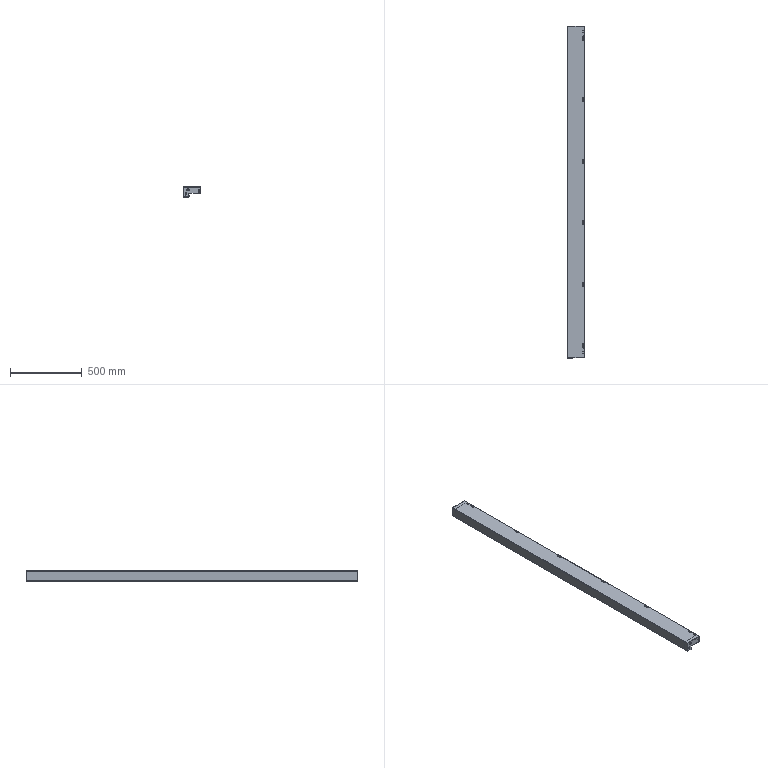Part | 3 solids | 230 faces | box 120 x 2316 x 70 mm | volume 834550 mm3 | plane 142 | cylinder 88 | commonest cylinder face diameters 6.2 x28 9 x18 11 x10 3.4 x9 4 x8 8 x6